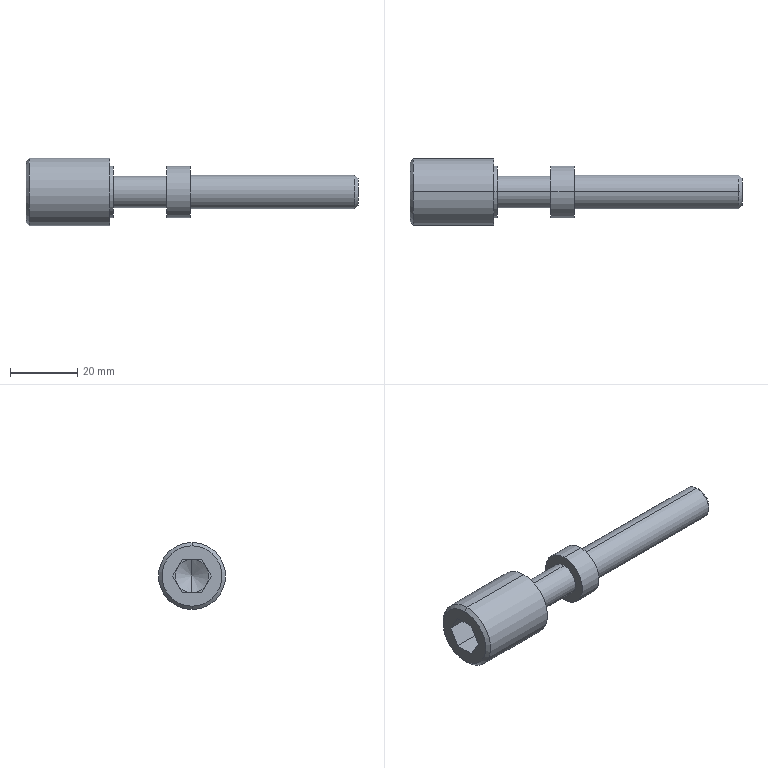Part | STEP file | AJKTN10-50 adjusting screw | 1 solid | 34 faces | box 99 x 20 x 20 mm | volume 13265 mm3 | plane 18 | cylinder 10 | cone 6 | commonest cylinder face diameters 15.5 x4 9.5 x2 10 x2 20 x2